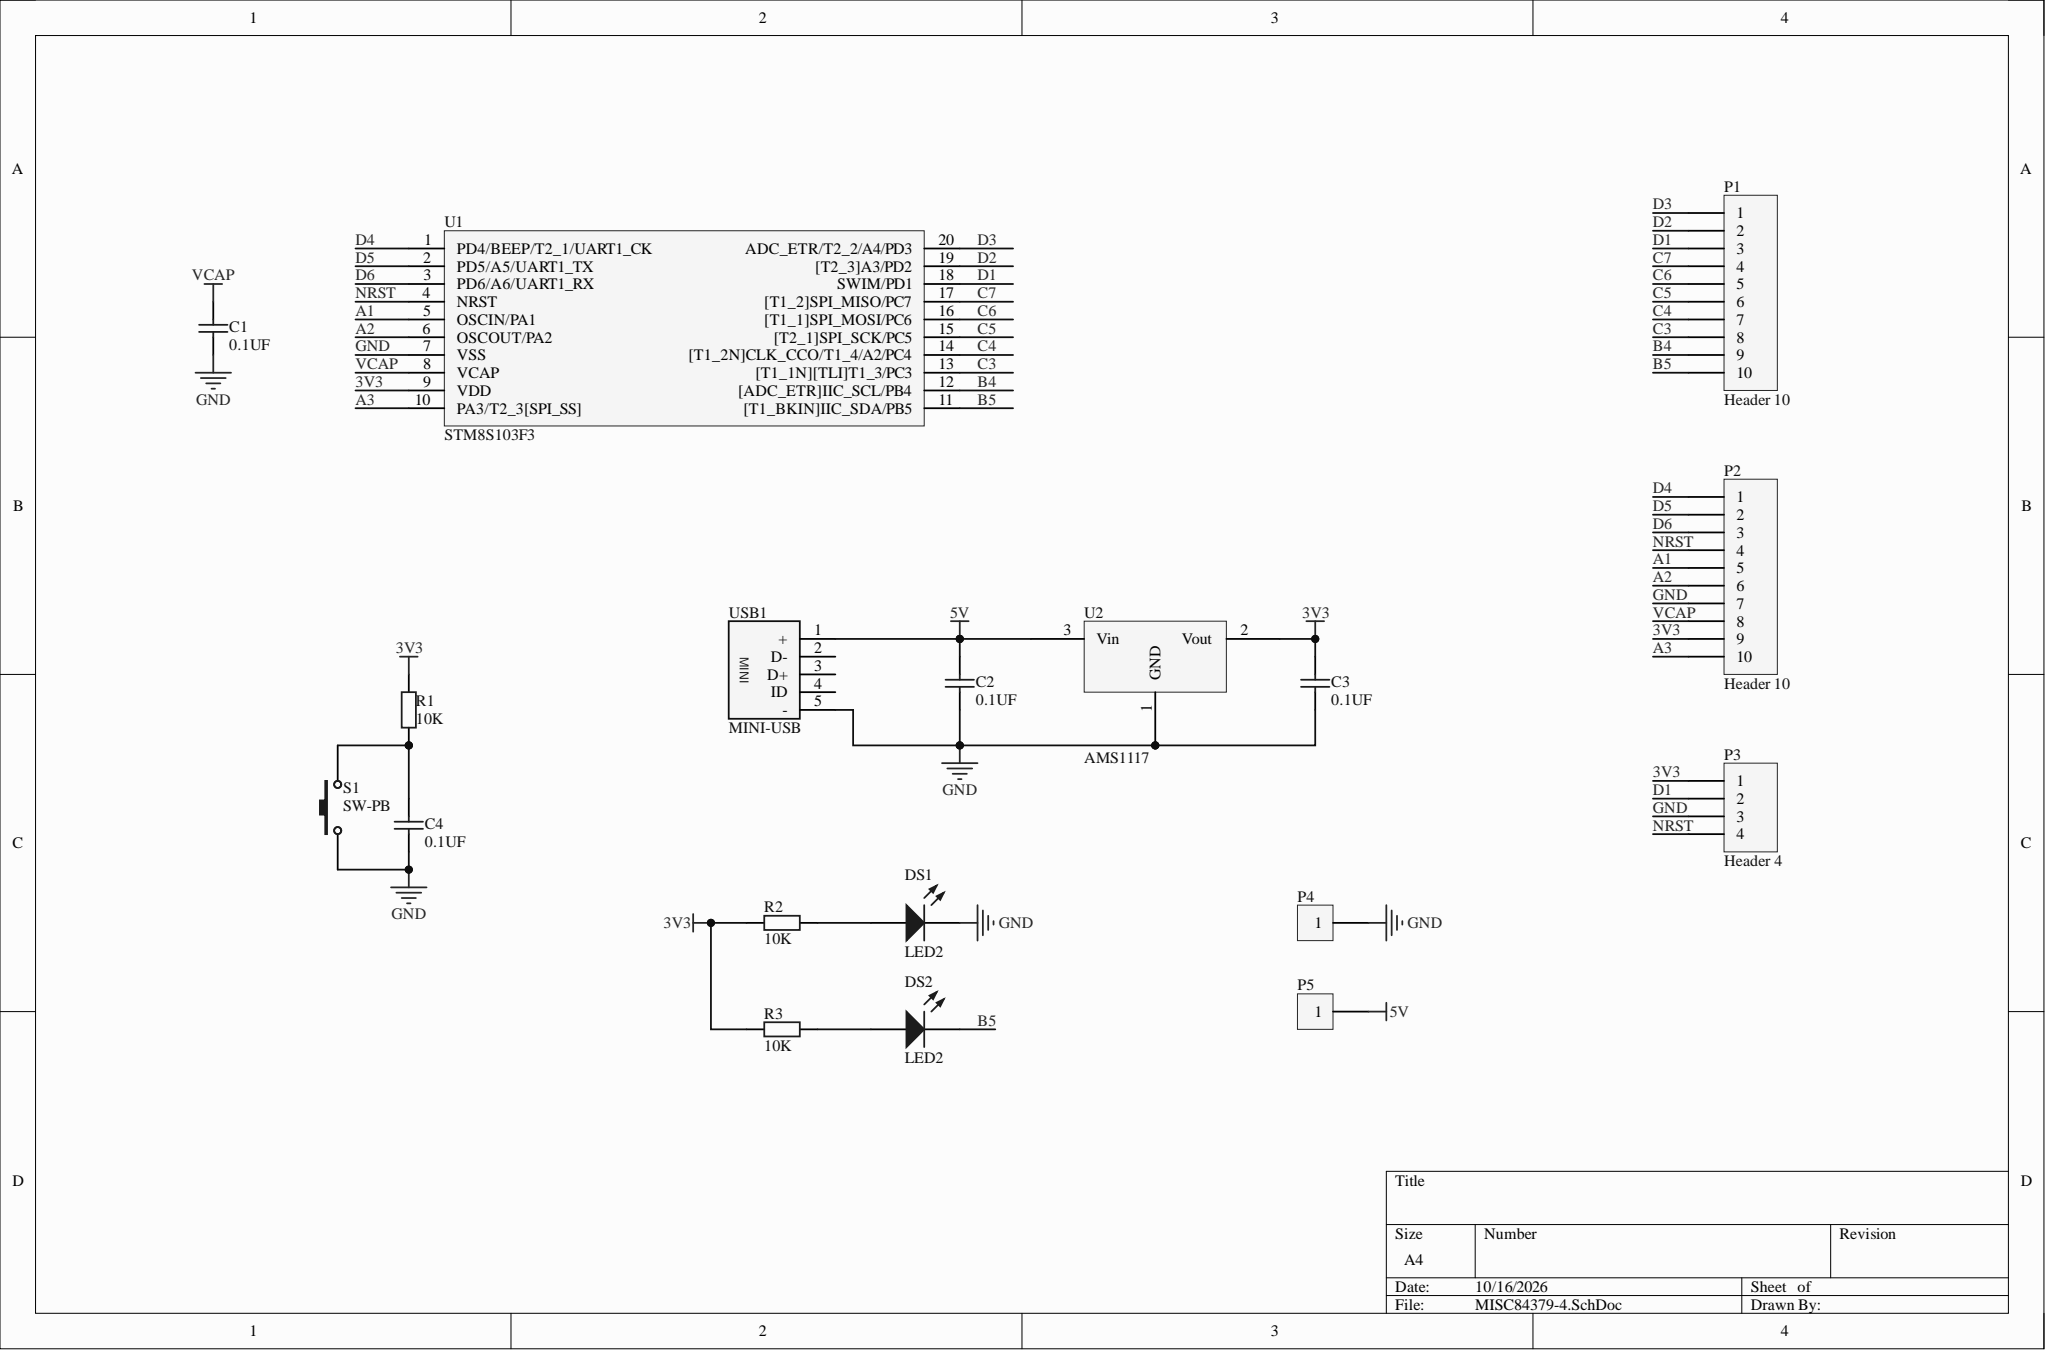Circuit board | Altium Designer | 18 parts | 24 nets
Bill of materials:
Comment,Description,Designator,Footprint,LibRef,Quantity
"0.1UF","Capacitor (Semiconductor SIM Model)","C1, C2, C3, C4","C1206","Cap Semi","4"
"LED2","Typical RED, GREEN, YELLOW, AMBER GaAs LED","DS1, DS2","my0603LED","LED2","2"
"Header 10","Header, 10-Pin","P1, P2","HDR1X10","Header 10","2"
"Header 4","Header, 4-Pin","P3","HDR1X4","Header 4","1"
"HDR1X1","","P4, P5","HDR1X1","HDR1X1","2"
"Res2","Resistor","R1, R2, R3","my0603","Res2","3"
"SW-PB","Switch","S1","SW_PB2_A1","SW-PB","1"
"STM8S103F3","","U1","SOP-20","STM8S103F3","1"
"AMS1117","Three-terminal regulator IC","U2","SOT223","AMS1117","1"
"MINI-USB","","USB1","USB-MINI-A","MINI-USB","1"
Netlist (Protel format):
[
C1
C1206
0.1UF



]
[
C2
C1206
0.1UF



]
[
C3
C1206
0.1UF



]
[
C4
C1206
0.1UF



]
[
DS1
my0603LED
LED2



]
[
DS2
my0603LED
LED2



]
[
P1
HDR1X10
Header 10



]
[
P2
HDR1X10
Header 10



]
[
P3
HDR1X4
Header 4



]
[
P4
HDR1X1
HDR1X1



]
[
P5
HDR1X1
HDR1X1



]
[
R1
my0603
Res2



]
[
R2
my0603
Res2



]
[
R3
my0603
Res2



]
[
S1
SW_PB2_A1
SW-PB



]
[
U1
SOP-20
STM8S103F3



]
[
U2
SOT223
AMS1117



]
[
USB1
USB-MINI-A
MINI-USB



]
(
VCAP
C1-2
P2-8
U1-8
)
(
NRST
P2-4
P3-4
U1-4
)
(
NetDS2_1
DS2-1
R3-1
)
(
NetDS1_1
DS1-1
R2-1
)
(
NetC4_2
C4-2
R1-1
S1-2
)
(
GND
C1-1
C2-1
C3-1
C4-1
DS1-2
P2-7
P3-3
P4-1
S1-1
U1-7
U2-1
USB1-5
)
(
D6
P2-3
U1-3
)
(
D5
P2-2
U1-2
)
(
D4
P2-1
U1-1
)
(
D3
P1-1
U1-20
)
(
D2
P1-2
U1-19
)
(
D1
P1-3
P3-2
U1-18
)
(
C7
P1-4
U1-17
)
(
C6
P1-5
U1-16
)
(
C5
P1-6
U1-15
)
(
C4
P1-7
U1-14
)
(
C3
P1-8
U1-13
)
(
B5
DS2-2
P1-10
U1-11
)
(
B4
P1-9
U1-12
)
(
A3
P2-10
U1-10
)
(
A2
P2-6
U1-6
)
(
A1
P2-5
U1-5
)
(
5V
C2-2
P5-1
U2-3
USB1-1
)
(
3V3
C3-2
P2-9
P3-1
R1-2
R2-2
R3-2
U1-9
U2-2
)